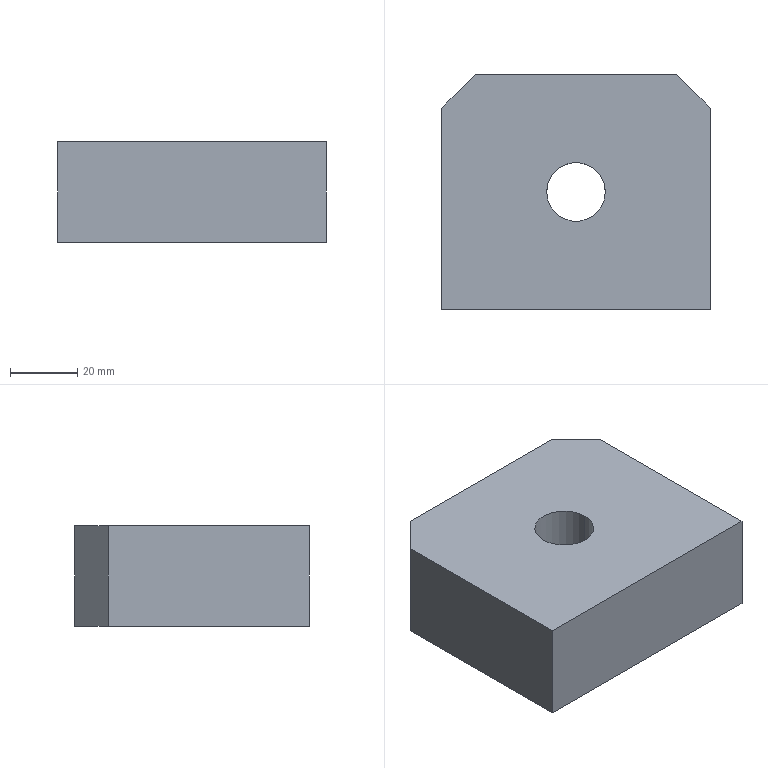Part | STEP file | Thickening Block | 1 solid | 10 faces | box 80 x 70 x 30 mm | volume 157784 mm3 | plane 8 | cylinder 2 | commonest cylinder face diameters 17.5 x2
STEP:
#1=CARTESIAN_POINT('',(0.,0.,0.));
#2=DIRECTION('',(0.,0.,1.));
#3=DIRECTION('',(1.,0.,0.));
#4=AXIS2_PLACEMENT_3D('',#1,#2,#3);
#5=CARTESIAN_POINT('',(8.75,0.,0.));
#6=VERTEX_POINT('',#5);
#7=CARTESIAN_POINT('',(8.75,0.,30.));
#8=VERTEX_POINT('',#7);
#9=CARTESIAN_POINT('',(8.75,0.,30.));
#10=DIRECTION('',(0.,0.,1.));
#11=VECTOR('',#10,1.);
#12=LINE('',#9,#11);
#13=CARTESIAN_POINT('',(0.,0.,30.));
#14=DIRECTION('',(0.,0.,1.));
#15=DIRECTION('',(1.,0.,0.));
#16=AXIS2_PLACEMENT_3D('',#13,#14,#15);
#17=CYLINDRICAL_SURFACE('',#16,8.75);
#18=CARTESIAN_POINT('',(6.283,0.));
#19=DIRECTION('',(0.,1.));
#20=VECTOR('',#19,1.);
#21=LINE('',#18,#20);
#22=(GEOMETRIC_REPRESENTATION_CONTEXT(2)PARAMETRIC_REPRESENTATION_CONTEXT()REPRESENTATION_CONTEXT('',''));
#23=DEFINITIONAL_REPRESENTATION('',(#21),#22);
#24=PCURVE('',#17,#23);
#25=CARTESIAN_POINT('',(0.,0.,30.));
#26=DIRECTION('',(0.,0.,1.));
#27=DIRECTION('',(1.,0.,0.));
#28=AXIS2_PLACEMENT_3D('',#25,#26,#27);
#29=CYLINDRICAL_SURFACE('',#28,8.75);
#30=CARTESIAN_POINT('',(0.,0.));
#31=DIRECTION('',(0.,1.));
#32=VECTOR('',#31,1.);
#33=LINE('',#30,#32);
#34=(GEOMETRIC_REPRESENTATION_CONTEXT(2)PARAMETRIC_REPRESENTATION_CONTEXT()REPRESENTATION_CONTEXT('',''));
#35=DEFINITIONAL_REPRESENTATION('',(#33),#34);
#36=PCURVE('',#29,#35);
#37=SURFACE_CURVE('',#12,(#24,#36),.PCURVE_S1.);
#38=EDGE_CURVE('',#6,#8,#37,.T.);
#39=ORIENTED_EDGE('',*,*,#38,.T.);
#40=CARTESIAN_POINT('',(-8.75,0.,30.));
#41=VERTEX_POINT('',#40);
#42=CARTESIAN_POINT('',(0.,0.,30.));
#43=DIRECTION('',(0.,0.,1.));
#44=DIRECTION('',(1.,0.,0.));
#45=AXIS2_PLACEMENT_3D('',#42,#43,#44);
#46=CIRCLE('',#45,8.75);
#47=CARTESIAN_POINT('',(0.,0.));
#48=DIRECTION('',(1.,0.));
#49=VECTOR('',#48,1.);
#50=LINE('',#47,#49);
#51=(GEOMETRIC_REPRESENTATION_CONTEXT(2)PARAMETRIC_REPRESENTATION_CONTEXT()REPRESENTATION_CONTEXT('',''));
#52=DEFINITIONAL_REPRESENTATION('',(#50),#51);
#53=PCURVE('',#17,#52);
#54=CARTESIAN_POINT('',(0.,0.,30.));
#55=DIRECTION('',(0.,0.,1.));
#56=DIRECTION('',(1.,0.,0.));
#57=AXIS2_PLACEMENT_3D('',#54,#55,#56);
#58=PLANE('',#57);
#59=CARTESIAN_POINT('',(0.,0.));
#60=DIRECTION('',(1.,0.));
#61=AXIS2_PLACEMENT_2D('',#59,#60);
#62=CIRCLE('',#61,8.75);
#63=(GEOMETRIC_REPRESENTATION_CONTEXT(2)PARAMETRIC_REPRESENTATION_CONTEXT()REPRESENTATION_CONTEXT('',''));
#64=DEFINITIONAL_REPRESENTATION('',(#62),#63);
#65=PCURVE('',#58,#64);
#66=SURFACE_CURVE('',#46,(#53,#65),.PCURVE_S1.);
#67=EDGE_CURVE('',#41,#8,#66,.T.);
#68=ORIENTED_EDGE('',*,*,#67,.F.);
#69=CARTESIAN_POINT('',(-8.75,0.,0.));
#70=VERTEX_POINT('',#69);
#71=CARTESIAN_POINT('',(-8.75,0.,30.));
#72=DIRECTION('',(0.,0.,1.));
#73=VECTOR('',#72,1.);
#74=LINE('',#71,#73);
#75=CARTESIAN_POINT('',(3.142,0.));
#76=DIRECTION('',(0.,1.));
#77=VECTOR('',#76,1.);
#78=LINE('',#75,#77);
#79=(GEOMETRIC_REPRESENTATION_CONTEXT(2)PARAMETRIC_REPRESENTATION_CONTEXT()REPRESENTATION_CONTEXT('',''));
#80=DEFINITIONAL_REPRESENTATION('',(#78),#79);
#81=PCURVE('',#17,#80);
#82=CARTESIAN_POINT('',(3.142,0.));
#83=DIRECTION('',(0.,1.));
#84=VECTOR('',#83,1.);
#85=LINE('',#82,#84);
#86=(GEOMETRIC_REPRESENTATION_CONTEXT(2)PARAMETRIC_REPRESENTATION_CONTEXT()REPRESENTATION_CONTEXT('',''));
#87=DEFINITIONAL_REPRESENTATION('',(#85),#86);
#88=PCURVE('',#29,#87);
#89=SURFACE_CURVE('',#74,(#81,#88),.PCURVE_S1.);
#90=EDGE_CURVE('',#70,#41,#89,.T.);
#91=ORIENTED_EDGE('',*,*,#90,.F.);
#92=CARTESIAN_POINT('',(0.,0.,0.));
#93=DIRECTION('',(0.,0.,1.));
#94=DIRECTION('',(1.,0.,0.));
#95=AXIS2_PLACEMENT_3D('',#92,#93,#94);
#96=CIRCLE('',#95,8.75);
#97=CARTESIAN_POINT('',(0.,-30.));
#98=DIRECTION('',(1.,0.));
#99=VECTOR('',#98,1.);
#100=LINE('',#97,#99);
#101=(GEOMETRIC_REPRESENTATION_CONTEXT(2)PARAMETRIC_REPRESENTATION_CONTEXT()REPRESENTATION_CONTEXT('',''));
#102=DEFINITIONAL_REPRESENTATION('',(#100),#101);
#103=PCURVE('',#17,#102);
#104=CARTESIAN_POINT('',(0.,0.,0.));
#105=DIRECTION('',(0.,0.,1.));
#106=DIRECTION('',(1.,0.,0.));
#107=AXIS2_PLACEMENT_3D('',#104,#105,#106);
#108=PLANE('',#107);
#109=CARTESIAN_POINT('',(0.,0.));
#110=DIRECTION('',(1.,0.));
#111=AXIS2_PLACEMENT_2D('',#109,#110);
#112=CIRCLE('',#111,8.75);
#113=(GEOMETRIC_REPRESENTATION_CONTEXT(2)PARAMETRIC_REPRESENTATION_CONTEXT()REPRESENTATION_CONTEXT('',''));
#114=DEFINITIONAL_REPRESENTATION('',(#112),#113);
#115=PCURVE('',#108,#114);
#116=SURFACE_CURVE('',#96,(#103,#115),.PCURVE_S1.);
#117=EDGE_CURVE('',#70,#6,#116,.T.);
#118=ORIENTED_EDGE('',*,*,#117,.T.);
#119=EDGE_LOOP('',(#39,#68,#91,#118));
#120=FACE_BOUND('',#119,.F.);
#121=ADVANCED_FACE('',(#120),#17,.F.);
#122=CARTESIAN_POINT('',(40.,-35.,0.));
#123=VERTEX_POINT('',#122);
#124=CARTESIAN_POINT('',(40.,25.,0.));
#125=VERTEX_POINT('',#124);
#126=CARTESIAN_POINT('',(40.,35.,0.));
#127=DIRECTION('',(0.,1.,0.));
#128=VECTOR('',#127,1.);
#129=LINE('',#126,#128);
#130=CARTESIAN_POINT('',(40.,35.,30.));
#131=DIRECTION('',(-1.,0.,0.));
#132=DIRECTION('',(0.,-1.,0.));
#133=AXIS2_PLACEMENT_3D('',#130,#131,#132);
#134=PLANE('',#133);
#135=CARTESIAN_POINT('',(0.,-30.));
#136=DIRECTION('',(-1.,0.));
#137=VECTOR('',#136,1.);
#138=LINE('',#135,#137);
#139=(GEOMETRIC_REPRESENTATION_CONTEXT(2)PARAMETRIC_REPRESENTATION_CONTEXT()REPRESENTATION_CONTEXT('',''));
#140=DEFINITIONAL_REPRESENTATION('',(#138),#139);
#141=PCURVE('',#134,#140);
#142=CARTESIAN_POINT('',(40.,35.));
#143=DIRECTION('',(0.,1.));
#144=VECTOR('',#143,1.);
#145=LINE('',#142,#144);
#146=(GEOMETRIC_REPRESENTATION_CONTEXT(2)PARAMETRIC_REPRESENTATION_CONTEXT()REPRESENTATION_CONTEXT('',''));
#147=DEFINITIONAL_REPRESENTATION('',(#145),#146);
#148=PCURVE('',#108,#147);
#149=SURFACE_CURVE('',#129,(#141,#148),.PCURVE_S1.);
#150=EDGE_CURVE('',#123,#125,#149,.T.);
#151=ORIENTED_EDGE('',*,*,#150,.T.);
#152=CARTESIAN_POINT('',(40.,25.,30.));
#153=VERTEX_POINT('',#152);
#154=CARTESIAN_POINT('',(40.,25.,30.));
#155=DIRECTION('',(0.,0.,1.));
#156=VECTOR('',#155,1.);
#157=LINE('',#154,#156);
#158=CARTESIAN_POINT('',(10.,0.));
#159=DIRECTION('',(0.,1.));
#160=VECTOR('',#159,1.);
#161=LINE('',#158,#160);
#162=(GEOMETRIC_REPRESENTATION_CONTEXT(2)PARAMETRIC_REPRESENTATION_CONTEXT()REPRESENTATION_CONTEXT('',''));
#163=DEFINITIONAL_REPRESENTATION('',(#161),#162);
#164=PCURVE('',#134,#163);
#165=CARTESIAN_POINT('',(30.,35.,30.));
#166=DIRECTION('',(-0.7071,-0.7071,0.));
#167=DIRECTION('',(0.,0.,-1.));
#168=AXIS2_PLACEMENT_3D('',#165,#166,#167);
#169=PLANE('',#168);
#170=CARTESIAN_POINT('',(0.,14.142));
#171=DIRECTION('',(-1.,0.));
#172=VECTOR('',#171,1.);
#173=LINE('',#170,#172);
#174=(GEOMETRIC_REPRESENTATION_CONTEXT(2)PARAMETRIC_REPRESENTATION_CONTEXT()REPRESENTATION_CONTEXT('',''));
#175=DEFINITIONAL_REPRESENTATION('',(#173),#174);
#176=PCURVE('',#169,#175);
#177=SURFACE_CURVE('',#157,(#164,#176),.PCURVE_S1.);
#178=EDGE_CURVE('',#125,#153,#177,.T.);
#179=ORIENTED_EDGE('',*,*,#178,.T.);
#180=CARTESIAN_POINT('',(40.,-35.,30.));
#181=VERTEX_POINT('',#180);
#182=CARTESIAN_POINT('',(40.,35.,30.));
#183=DIRECTION('',(0.,1.,0.));
#184=VECTOR('',#183,1.);
#185=LINE('',#182,#184);
#186=CARTESIAN_POINT('',(0.,0.));
#187=DIRECTION('',(-1.,0.));
#188=VECTOR('',#187,1.);
#189=LINE('',#186,#188);
#190=(GEOMETRIC_REPRESENTATION_CONTEXT(2)PARAMETRIC_REPRESENTATION_CONTEXT()REPRESENTATION_CONTEXT('',''));
#191=DEFINITIONAL_REPRESENTATION('',(#189),#190);
#192=PCURVE('',#134,#191);
#193=CARTESIAN_POINT('',(40.,35.));
#194=DIRECTION('',(0.,1.));
#195=VECTOR('',#194,1.);
#196=LINE('',#193,#195);
#197=(GEOMETRIC_REPRESENTATION_CONTEXT(2)PARAMETRIC_REPRESENTATION_CONTEXT()REPRESENTATION_CONTEXT('',''));
#198=DEFINITIONAL_REPRESENTATION('',(#196),#197);
#199=PCURVE('',#58,#198);
#200=SURFACE_CURVE('',#185,(#192,#199),.PCURVE_S1.);
#201=EDGE_CURVE('',#181,#153,#200,.T.);
#202=ORIENTED_EDGE('',*,*,#201,.F.);
#203=CARTESIAN_POINT('',(40.,-35.,30.));
#204=DIRECTION('',(0.,0.,-1.));
#205=VECTOR('',#204,1.);
#206=LINE('',#203,#205);
#207=CARTESIAN_POINT('',(70.,0.));
#208=DIRECTION('',(0.,-1.));
#209=VECTOR('',#208,1.);
#210=LINE('',#207,#209);
#211=(GEOMETRIC_REPRESENTATION_CONTEXT(2)PARAMETRIC_REPRESENTATION_CONTEXT()REPRESENTATION_CONTEXT('',''));
#212=DEFINITIONAL_REPRESENTATION('',(#210),#211);
#213=PCURVE('',#134,#212);
#214=CARTESIAN_POINT('',(-40.,-35.,30.));
#215=DIRECTION('',(0.,1.,0.));
#216=DIRECTION('',(0.,0.,1.));
#217=AXIS2_PLACEMENT_3D('',#214,#215,#216);
#218=PLANE('',#217);
#219=CARTESIAN_POINT('',(0.,80.));
#220=DIRECTION('',(-1.,0.));
#221=VECTOR('',#220,1.);
#222=LINE('',#219,#221);
#223=(GEOMETRIC_REPRESENTATION_CONTEXT(2)PARAMETRIC_REPRESENTATION_CONTEXT()REPRESENTATION_CONTEXT('',''));
#224=DEFINITIONAL_REPRESENTATION('',(#222),#223);
#225=PCURVE('',#218,#224);
#226=SURFACE_CURVE('',#206,(#213,#225),.PCURVE_S1.);
#227=EDGE_CURVE('',#181,#123,#226,.T.);
#228=ORIENTED_EDGE('',*,*,#227,.T.);
#229=EDGE_LOOP('',(#151,#179,#202,#228));
#230=FACE_BOUND('',#229,.T.);
#231=ADVANCED_FACE('',(#230),#134,.F.);
#232=CARTESIAN_POINT('',(30.,35.,30.));
#233=VERTEX_POINT('',#232);
#234=CARTESIAN_POINT('',(-30.,35.,30.));
#235=VERTEX_POINT('',#234);
#236=CARTESIAN_POINT('',(-40.,35.,30.));
#237=DIRECTION('',(-1.,0.,0.));
#238=VECTOR('',#237,1.);
#239=LINE('',#236,#238);
#240=CARTESIAN_POINT('',(-40.,35.,30.));
#241=DIRECTION('',(0.,-1.,0.));
#242=DIRECTION('',(0.,0.,-1.));
#243=AXIS2_PLACEMENT_3D('',#240,#241,#242);
#244=PLANE('',#243);
#245=CARTESIAN_POINT('',(0.,0.));
#246=DIRECTION('',(0.,-1.));
#247=VECTOR('',#246,1.);
#248=LINE('',#245,#247);
#249=(GEOMETRIC_REPRESENTATION_CONTEXT(2)PARAMETRIC_REPRESENTATION_CONTEXT()REPRESENTATION_CONTEXT('',''));
#250=DEFINITIONAL_REPRESENTATION('',(#248),#249);
#251=PCURVE('',#244,#250);
#252=CARTESIAN_POINT('',(-40.,35.));
#253=DIRECTION('',(-1.,0.));
#254=VECTOR('',#253,1.);
#255=LINE('',#252,#254);
#256=(GEOMETRIC_REPRESENTATION_CONTEXT(2)PARAMETRIC_REPRESENTATION_CONTEXT()REPRESENTATION_CONTEXT('',''));
#257=DEFINITIONAL_REPRESENTATION('',(#255),#256);
#258=PCURVE('',#58,#257);
#259=SURFACE_CURVE('',#239,(#251,#258),.PCURVE_S1.);
#260=EDGE_CURVE('',#233,#235,#259,.T.);
#261=ORIENTED_EDGE('',*,*,#260,.F.);
#262=CARTESIAN_POINT('',(30.,35.,0.));
#263=VERTEX_POINT('',#262);
#264=CARTESIAN_POINT('',(30.,35.,30.));
#265=DIRECTION('',(0.,0.,-1.));
#266=VECTOR('',#265,1.);
#267=LINE('',#264,#266);
#268=CARTESIAN_POINT('',(0.,70.));
#269=DIRECTION('',(1.,0.));
#270=VECTOR('',#269,1.);
#271=LINE('',#268,#270);
#272=(GEOMETRIC_REPRESENTATION_CONTEXT(2)PARAMETRIC_REPRESENTATION_CONTEXT()REPRESENTATION_CONTEXT('',''));
#273=DEFINITIONAL_REPRESENTATION('',(#271),#272);
#274=PCURVE('',#244,#273);
#275=CARTESIAN_POINT('',(0.,0.));
#276=DIRECTION('',(1.,0.));
#277=VECTOR('',#276,1.);
#278=LINE('',#275,#277);
#279=(GEOMETRIC_REPRESENTATION_CONTEXT(2)PARAMETRIC_REPRESENTATION_CONTEXT()REPRESENTATION_CONTEXT('',''));
#280=DEFINITIONAL_REPRESENTATION('',(#278),#279);
#281=PCURVE('',#169,#280);
#282=SURFACE_CURVE('',#267,(#274,#281),.PCURVE_S1.);
#283=EDGE_CURVE('',#233,#263,#282,.T.);
#284=ORIENTED_EDGE('',*,*,#283,.T.);
#285=CARTESIAN_POINT('',(-30.,35.,0.));
#286=VERTEX_POINT('',#285);
#287=CARTESIAN_POINT('',(-40.,35.,0.));
#288=DIRECTION('',(-1.,0.,0.));
#289=VECTOR('',#288,1.);
#290=LINE('',#287,#289);
#291=CARTESIAN_POINT('',(30.,0.));
#292=DIRECTION('',(0.,-1.));
#293=VECTOR('',#292,1.);
#294=LINE('',#291,#293);
#295=(GEOMETRIC_REPRESENTATION_CONTEXT(2)PARAMETRIC_REPRESENTATION_CONTEXT()REPRESENTATION_CONTEXT('',''));
#296=DEFINITIONAL_REPRESENTATION('',(#294),#295);
#297=PCURVE('',#244,#296);
#298=CARTESIAN_POINT('',(-40.,35.));
#299=DIRECTION('',(-1.,0.));
#300=VECTOR('',#299,1.);
#301=LINE('',#298,#300);
#302=(GEOMETRIC_REPRESENTATION_CONTEXT(2)PARAMETRIC_REPRESENTATION_CONTEXT()REPRESENTATION_CONTEXT('',''));
#303=DEFINITIONAL_REPRESENTATION('',(#301),#302);
#304=PCURVE('',#108,#303);
#305=SURFACE_CURVE('',#290,(#297,#304),.PCURVE_S1.);
#306=EDGE_CURVE('',#263,#286,#305,.T.);
#307=ORIENTED_EDGE('',*,*,#306,.T.);
#308=CARTESIAN_POINT('',(-30.,35.,30.));
#309=DIRECTION('',(0.,0.,1.));
#310=VECTOR('',#309,1.);
#311=LINE('',#308,#310);
#312=CARTESIAN_POINT('',(0.,10.));
#313=DIRECTION('',(-1.,0.));
#314=VECTOR('',#313,1.);
#315=LINE('',#312,#314);
#316=(GEOMETRIC_REPRESENTATION_CONTEXT(2)PARAMETRIC_REPRESENTATION_CONTEXT()REPRESENTATION_CONTEXT('',''));
#317=DEFINITIONAL_REPRESENTATION('',(#315),#316);
#318=PCURVE('',#244,#317);
#319=CARTESIAN_POINT('',(-40.,25.,30.));
#320=DIRECTION('',(0.7071,-0.7071,0.));
#321=DIRECTION('',(0.,0.,-1.));
#322=AXIS2_PLACEMENT_3D('',#319,#320,#321);
#323=PLANE('',#322);
#324=CARTESIAN_POINT('',(0.,14.142));
#325=DIRECTION('',(-1.,0.));
#326=VECTOR('',#325,1.);
#327=LINE('',#324,#326);
#328=(GEOMETRIC_REPRESENTATION_CONTEXT(2)PARAMETRIC_REPRESENTATION_CONTEXT()REPRESENTATION_CONTEXT('',''));
#329=DEFINITIONAL_REPRESENTATION('',(#327),#328);
#330=PCURVE('',#323,#329);
#331=SURFACE_CURVE('',#311,(#318,#330),.PCURVE_S1.);
#332=EDGE_CURVE('',#286,#235,#331,.T.);
#333=ORIENTED_EDGE('',*,*,#332,.T.);
#334=EDGE_LOOP('',(#261,#284,#307,#333));
#335=FACE_BOUND('',#334,.T.);
#336=ADVANCED_FACE('',(#335),#244,.F.);
#337=CARTESIAN_POINT('',(-40.,25.,30.));
#338=VERTEX_POINT('',#337);
#339=CARTESIAN_POINT('',(-40.,-35.,30.));
#340=VERTEX_POINT('',#339);
#341=CARTESIAN_POINT('',(-40.,35.,30.));
#342=DIRECTION('',(0.,-1.,0.));
#343=VECTOR('',#342,1.);
#344=LINE('',#341,#343);
#345=CARTESIAN_POINT('',(-40.,35.,30.));
#346=DIRECTION('',(1.,0.,0.));
#347=DIRECTION('',(0.,1.,0.));
#348=AXIS2_PLACEMENT_3D('',#345,#346,#347);
#349=PLANE('',#348);
#350=CARTESIAN_POINT('',(0.,0.));
#351=DIRECTION('',(-1.,0.));
#352=VECTOR('',#351,1.);
#353=LINE('',#350,#352);
#354=(GEOMETRIC_REPRESENTATION_CONTEXT(2)PARAMETRIC_REPRESENTATION_CONTEXT()REPRESENTATION_CONTEXT('',''));
#355=DEFINITIONAL_REPRESENTATION('',(#353),#354);
#356=PCURVE('',#349,#355);
#357=CARTESIAN_POINT('',(-40.,35.));
#358=DIRECTION('',(0.,-1.));
#359=VECTOR('',#358,1.);
#360=LINE('',#357,#359);
#361=(GEOMETRIC_REPRESENTATION_CONTEXT(2)PARAMETRIC_REPRESENTATION_CONTEXT()REPRESENTATION_CONTEXT('',''));
#362=DEFINITIONAL_REPRESENTATION('',(#360),#361);
#363=PCURVE('',#58,#362);
#364=SURFACE_CURVE('',#344,(#356,#363),.PCURVE_S1.);
#365=EDGE_CURVE('',#338,#340,#364,.T.);
#366=ORIENTED_EDGE('',*,*,#365,.F.);
#367=CARTESIAN_POINT('',(-40.,25.,0.));
#368=VERTEX_POINT('',#367);
#369=CARTESIAN_POINT('',(-40.,25.,30.));
#370=DIRECTION('',(0.,0.,-1.));
#371=VECTOR('',#370,1.);
#372=LINE('',#369,#371);
#373=CARTESIAN_POINT('',(-10.,0.));
#374=DIRECTION('',(0.,-1.));
#375=VECTOR('',#374,1.);
#376=LINE('',#373,#375);
#377=(GEOMETRIC_REPRESENTATION_CONTEXT(2)PARAMETRIC_REPRESENTATION_CONTEXT()REPRESENTATION_CONTEXT('',''));
#378=DEFINITIONAL_REPRESENTATION('',(#376),#377);
#379=PCURVE('',#349,#378);
#380=CARTESIAN_POINT('',(0.,0.));
#381=DIRECTION('',(1.,0.));
#382=VECTOR('',#381,1.);
#383=LINE('',#380,#382);
#384=(GEOMETRIC_REPRESENTATION_CONTEXT(2)PARAMETRIC_REPRESENTATION_CONTEXT()REPRESENTATION_CONTEXT('',''));
#385=DEFINITIONAL_REPRESENTATION('',(#383),#384);
#386=PCURVE('',#323,#385);
#387=SURFACE_CURVE('',#372,(#379,#386),.PCURVE_S1.);
#388=EDGE_CURVE('',#338,#368,#387,.T.);
#389=ORIENTED_EDGE('',*,*,#388,.T.);
#390=CARTESIAN_POINT('',(-40.,-35.,0.));
#391=VERTEX_POINT('',#390);
#392=CARTESIAN_POINT('',(-40.,35.,0.));
#393=DIRECTION('',(0.,-1.,0.));
#394=VECTOR('',#393,1.);
#395=LINE('',#392,#394);
#396=CARTESIAN_POINT('',(0.,-30.));
#397=DIRECTION('',(-1.,0.));
#398=VECTOR('',#397,1.);
#399=LINE('',#396,#398);
#400=(GEOMETRIC_REPRESENTATION_CONTEXT(2)PARAMETRIC_REPRESENTATION_CONTEXT()REPRESENTATION_CONTEXT('',''));
#401=DEFINITIONAL_REPRESENTATION('',(#399),#400);
#402=PCURVE('',#349,#401);
#403=CARTESIAN_POINT('',(-40.,35.));
#404=DIRECTION('',(0.,-1.));
#405=VECTOR('',#404,1.);
#406=LINE('',#403,#405);
#407=(GEOMETRIC_REPRESENTATION_CONTEXT(2)PARAMETRIC_REPRESENTATION_CONTEXT()REPRESENTATION_CONTEXT('',''));
#408=DEFINITIONAL_REPRESENTATION('',(#406),#407);
#409=PCURVE('',#108,#408);
#410=SURFACE_CURVE('',#395,(#402,#409),.PCURVE_S1.);
#411=EDGE_CURVE('',#368,#391,#410,.T.);
#412=ORIENTED_EDGE('',*,*,#411,.T.);
#413=CARTESIAN_POINT('',(-40.,-35.,30.));
#414=DIRECTION('',(0.,0.,-1.));
#415=VECTOR('',#414,1.);
#416=LINE('',#413,#415);
#417=CARTESIAN_POINT('',(-70.,0.));
#418=DIRECTION('',(0.,-1.));
#419=VECTOR('',#418,1.);
#420=LINE('',#417,#419);
#421=(GEOMETRIC_REPRESENTATION_CONTEXT(2)PARAMETRIC_REPRESENTATION_CONTEXT()REPRESENTATION_CONTEXT('',''));
#422=DEFINITIONAL_REPRESENTATION('',(#420),#421);
#423=PCURVE('',#349,#422);
#424=CARTESIAN_POINT('',(0.,0.));
#425=DIRECTION('',(-1.,0.));
#426=VECTOR('',#425,1.);
#427=LINE('',#424,#426);
#428=(GEOMETRIC_REPRESENTATION_CONTEXT(2)PARAMETRIC_REPRESENTATION_CONTEXT()REPRESENTATION_CONTEXT('',''));
#429=DEFINITIONAL_REPRESENTATION('',(#427),#428);
#430=PCURVE('',#218,#429);
#431=SURFACE_CURVE('',#416,(#423,#430),.PCURVE_S1.);
#432=EDGE_CURVE('',#340,#391,#431,.T.);
#433=ORIENTED_EDGE('',*,*,#432,.F.);
#434=EDGE_LOOP('',(#366,#389,#412,#433));
#435=FACE_BOUND('',#434,.T.);
#436=ADVANCED_FACE('',(#435),#349,.F.);
#437=CARTESIAN_POINT('',(-40.,-35.,0.));
#438=DIRECTION('',(1.,0.,0.));
#439=VECTOR('',#438,1.);
#440=LINE('',#437,#439);
#441=CARTESIAN_POINT('',(-30.,0.));
#442=DIRECTION('',(0.,1.));
#443=VECTOR('',#442,1.);
#444=LINE('',#441,#443);
#445=(GEOMETRIC_REPRESENTATION_CONTEXT(2)PARAMETRIC_REPRESENTATION_CONTEXT()REPRESENTATION_CONTEXT('',''));
#446=DEFINITIONAL_REPRESENTATION('',(#444),#445);
#447=PCURVE('',#218,#446);
#448=CARTESIAN_POINT('',(-40.,-35.));
#449=DIRECTION('',(1.,0.));
#450=VECTOR('',#449,1.);
#451=LINE('',#448,#450);
#452=(GEOMETRIC_REPRESENTATION_CONTEXT(2)PARAMETRIC_REPRESENTATION_CONTEXT()REPRESENTATION_CONTEXT('',''));
#453=DEFINITIONAL_REPRESENTATION('',(#451),#452);
#454=PCURVE('',#108,#453);
#455=SURFACE_CURVE('',#440,(#447,#454),.PCURVE_S1.);
#456=EDGE_CURVE('',#391,#123,#455,.T.);
#457=ORIENTED_EDGE('',*,*,#456,.T.);
#458=ORIENTED_EDGE('',*,*,#227,.F.);
#459=CARTESIAN_POINT('',(-40.,-35.,30.));
#460=DIRECTION('',(1.,0.,0.));
#461=VECTOR('',#460,1.);
#462=LINE('',#459,#461);
#463=CARTESIAN_POINT('',(0.,0.));
#464=DIRECTION('',(0.,1.));
#465=VECTOR('',#464,1.);
#466=LINE('',#463,#465);
#467=(GEOMETRIC_REPRESENTATION_CONTEXT(2)PARAMETRIC_REPRESENTATION_CONTEXT()REPRESENTATION_CONTEXT('',''));
#468=DEFINITIONAL_REPRESENTATION('',(#466),#467);
#469=PCURVE('',#218,#468);
#470=CARTESIAN_POINT('',(-40.,-35.));
#471=DIRECTION('',(1.,0.));
#472=VECTOR('',#471,1.);
#473=LINE('',#470,#472);
#474=(GEOMETRIC_REPRESENTATION_CONTEXT(2)PARAMETRIC_REPRESENTATION_CONTEXT()REPRESENTATION_CONTEXT('',''));
#475=DEFINITIONAL_REPRESENTATION('',(#473),#474);
#476=PCURVE('',#58,#475);
#477=SURFACE_CURVE('',#462,(#469,#476),.PCURVE_S1.);
#478=EDGE_CURVE('',#340,#181,#477,.T.);
#479=ORIENTED_EDGE('',*,*,#478,.F.);
#480=ORIENTED_EDGE('',*,*,#432,.T.);
#481=EDGE_LOOP('',(#457,#458,#479,#480));
#482=FACE_BOUND('',#481,.T.);
#483=ADVANCED_FACE('',(#482),#218,.F.);
#484=CARTESIAN_POINT('',(0.,0.,30.));
#485=DIRECTION('',(0.,0.,1.));
#486=DIRECTION('',(1.,0.,0.));
#487=AXIS2_PLACEMENT_3D('',#484,#485,#486);
#488=CIRCLE('',#487,8.75);
#489=CARTESIAN_POINT('',(0.,0.));
#490=DIRECTION('',(1.,0.));
#491=AXIS2_PLACEMENT_2D('',#489,#490);
#492=CIRCLE('',#491,8.75);
#493=(GEOMETRIC_REPRESENTATION_CONTEXT(2)PARAMETRIC_REPRESENTATION_CONTEXT()REPRESENTATION_CONTEXT('',''));
#494=DEFINITIONAL_REPRESENTATION('',(#492),#493);
#495=PCURVE('',#58,#494);
#496=CARTESIAN_POINT('',(0.,0.));
#497=DIRECTION('',(1.,0.));
#498=VECTOR('',#497,1.);
#499=LINE('',#496,#498);
#500=(GEOMETRIC_REPRESENTATION_CONTEXT(2)PARAMETRIC_REPRESENTATION_CONTEXT()REPRESENTATION_CONTEXT('',''));
#501=DEFINITIONAL_REPRESENTATION('',(#499),#500);
#502=PCURVE('',#29,#501);
#503=SURFACE_CURVE('',#488,(#495,#502),.PCURVE_S1.);
#504=EDGE_CURVE('',#8,#41,#503,.T.);
#505=ORIENTED_EDGE('',*,*,#504,.F.);
#506=ORIENTED_EDGE('',*,*,#67,.F.);
#507=EDGE_LOOP('',(#505,#506));
#508=FACE_BOUND('',#507,.T.);
#509=ORIENTED_EDGE('',*,*,#201,.T.);
#510=CARTESIAN_POINT('',(32.5,32.5,30.));
#511=DIRECTION('',(-0.7071,0.7071,0.));
#512=VECTOR('',#511,1.);
#513=LINE('',#510,#512);
#514=CARTESIAN_POINT('',(32.5,32.5));
#515=DIRECTION('',(-0.7071,0.7071));
#516=VECTOR('',#515,1.);
#517=LINE('',#514,#516);
#518=(GEOMETRIC_REPRESENTATION_CONTEXT(2)PARAMETRIC_REPRESENTATION_CONTEXT()REPRESENTATION_CONTEXT('',''));
#519=DEFINITIONAL_REPRESENTATION('',(#517),#518);
#520=PCURVE('',#58,#519);
#521=CARTESIAN_POINT('',(0.,3.536));
#522=DIRECTION('',(0.,-1.));
#523=VECTOR('',#522,1.);
#524=LINE('',#521,#523);
#525=(GEOMETRIC_REPRESENTATION_CONTEXT(2)PARAMETRIC_REPRESENTATION_CONTEXT()REPRESENTATION_CONTEXT('',''));
#526=DEFINITIONAL_REPRESENTATION('',(#524),#525);
#527=PCURVE('',#169,#526);
#528=SURFACE_CURVE('',#513,(#520,#527),.PCURVE_S1.);
#529=EDGE_CURVE('',#153,#233,#528,.T.);
#530=ORIENTED_EDGE('',*,*,#529,.T.);
#531=ORIENTED_EDGE('',*,*,#260,.T.);
#532=CARTESIAN_POINT('',(-32.5,32.5,30.));
#533=DIRECTION('',(-0.7071,-0.7071,0.));
#534=VECTOR('',#533,1.);
#535=LINE('',#532,#534);
#536=CARTESIAN_POINT('',(-32.5,32.5));
#537=DIRECTION('',(-0.7071,-0.7071));
#538=VECTOR('',#537,1.);
#539=LINE('',#536,#538);
#540=(GEOMETRIC_REPRESENTATION_CONTEXT(2)PARAMETRIC_REPRESENTATION_CONTEXT()REPRESENTATION_CONTEXT('',''));
#541=DEFINITIONAL_REPRESENTATION('',(#539),#540);
#542=PCURVE('',#58,#541);
#543=CARTESIAN_POINT('',(0.,10.607));
#544=DIRECTION('',(0.,-1.));
#545=VECTOR('',#544,1.);
#546=LINE('',#543,#545);
#547=(GEOMETRIC_REPRESENTATION_CONTEXT(2)PARAMETRIC_REPRESENTATION_CONTEXT()REPRESENTATION_CONTEXT('',''));
#548=DEFINITIONAL_REPRESENTATION('',(#546),#547);
#549=PCURVE('',#323,#548);
#550=SURFACE_CURVE('',#535,(#542,#549),.PCURVE_S1.);
#551=EDGE_CURVE('',#235,#338,#550,.T.);
#552=ORIENTED_EDGE('',*,*,#551,.T.);
#553=ORIENTED_EDGE('',*,*,#365,.T.);
#554=ORIENTED_EDGE('',*,*,#478,.T.);
#555=EDGE_LOOP('',(#509,#530,#531,#552,#553,#554));
#556=FACE_BOUND('',#555,.T.);
#557=ADVANCED_FACE('',(#508,#556),#58,.T.);
#558=CARTESIAN_POINT('',(0.,0.,0.));
#559=DIRECTION('',(0.,0.,1.));
#560=DIRECTION('',(1.,0.,0.));
#561=AXIS2_PLACEMENT_3D('',#558,#559,#560);
#562=CIRCLE('',#561,8.75);
#563=CARTESIAN_POINT('',(0.,0.));
#564=DIRECTION('',(1.,0.));
#565=AXIS2_PLACEMENT_2D('',#563,#564);
#566=CIRCLE('',#565,8.75);
#567=(GEOMETRIC_REPRESENTATION_CONTEXT(2)PARAMETRIC_REPRESENTATION_CONTEXT()REPRESENTATION_CONTEXT('',''));
#568=DEFINITIONAL_REPRESENTATION('',(#566),#567);
#569=PCURVE('',#108,#568);
#570=CARTESIAN_POINT('',(0.,-30.));
#571=DIRECTION('',(1.,0.));
#572=VECTOR('',#571,1.);
#573=LINE('',#570,#572);
#574=(GEOMETRIC_REPRESENTATION_CONTEXT(2)PARAMETRIC_REPRESENTATION_CONTEXT()REPRESENTATION_CONTEXT('',''));
#575=DEFINITIONAL_REPRESENTATION('',(#573),#574);
#576=PCURVE('',#29,#575);
#577=SURFACE_CURVE('',#562,(#569,#576),.PCURVE_S1.);
#578=EDGE_CURVE('',#6,#70,#577,.T.);
#579=ORIENTED_EDGE('',*,*,#578,.T.);
#580=ORIENTED_EDGE('',*,*,#117,.T.);
#581=EDGE_LOOP('',(#579,#580));
#582=FACE_BOUND('',#581,.T.);
#583=ORIENTED_EDGE('',*,*,#306,.F.);
#584=CARTESIAN_POINT('',(30.,35.,0.));
#585=DIRECTION('',(0.7071,-0.7071,0.));
#586=VECTOR('',#585,1.);
#587=LINE('',#584,#586);
#588=CARTESIAN_POINT('',(30.,35.));
#589=DIRECTION('',(0.7071,-0.7071));
#590=VECTOR('',#589,1.);
#591=LINE('',#588,#590);
#592=(GEOMETRIC_REPRESENTATION_CONTEXT(2)PARAMETRIC_REPRESENTATION_CONTEXT()REPRESENTATION_CONTEXT('',''));
#593=DEFINITIONAL_REPRESENTATION('',(#591),#592);
#594=PCURVE('',#108,#593);
#595=CARTESIAN_POINT('',(30.,0.));
#596=DIRECTION('',(0.,1.));
#597=VECTOR('',#596,1.);
#598=LINE('',#595,#597);
#599=(GEOMETRIC_REPRESENTATION_CONTEXT(2)PARAMETRIC_REPRESENTATION_CONTEXT()REPRESENTATION_CONTEXT('',''));
#600=DEFINITIONAL_REPRESENTATION('',(#598),#599);
#601=PCURVE('',#169,#600);
#602=SURFACE_CURVE('',#587,(#594,#601),.PCURVE_S1.);
#603=EDGE_CURVE('',#263,#125,#602,.T.);
#604=ORIENTED_EDGE('',*,*,#603,.T.);
#605=ORIENTED_EDGE('',*,*,#150,.F.);
#606=ORIENTED_EDGE('',*,*,#456,.F.);
#607=ORIENTED_EDGE('',*,*,#411,.F.);
#608=CARTESIAN_POINT('',(-40.,25.,0.));
#609=DIRECTION('',(0.7071,0.7071,0.));
#610=VECTOR('',#609,1.);
#611=LINE('',#608,#610);
#612=CARTESIAN_POINT('',(-40.,25.));
#613=DIRECTION('',(0.7071,0.7071));
#614=VECTOR('',#613,1.);
#615=LINE('',#612,#614);
#616=(GEOMETRIC_REPRESENTATION_CONTEXT(2)PARAMETRIC_REPRESENTATION_CONTEXT()REPRESENTATION_CONTEXT('',''));
#617=DEFINITIONAL_REPRESENTATION('',(#615),#616);
#618=PCURVE('',#108,#617);
#619=CARTESIAN_POINT('',(30.,0.));
#620=DIRECTION('',(0.,1.));
#621=VECTOR('',#620,1.);
#622=LINE('',#619,#621);
#623=(GEOMETRIC_REPRESENTATION_CONTEXT(2)PARAMETRIC_REPRESENTATION_CONTEXT()REPRESENTATION_CONTEXT('',''));
#624=DEFINITIONAL_REPRESENTATION('',(#622),#623);
#625=PCURVE('',#323,#624);
#626=SURFACE_CURVE('',#611,(#618,#625),.PCURVE_S1.);
#627=EDGE_CURVE('',#368,#286,#626,.T.);
#628=ORIENTED_EDGE('',*,*,#627,.T.);
#629=EDGE_LOOP('',(#583,#604,#605,#606,#607,#628));
#630=FACE_BOUND('',#629,.T.);
#631=ADVANCED_FACE('',(#582,#630),#108,.F.);
#632=ORIENTED_EDGE('',*,*,#529,.F.);
#633=ORIENTED_EDGE('',*,*,#178,.F.);
#634=ORIENTED_EDGE('',*,*,#603,.F.);
#635=ORIENTED_EDGE('',*,*,#283,.F.);
#636=EDGE_LOOP('',(#632,#633,#634,#635));
#637=FACE_BOUND('',#636,.T.);
#638=ADVANCED_FACE('',(#637),#169,.F.);
#639=ORIENTED_EDGE('',*,*,#551,.F.);
#640=ORIENTED_EDGE('',*,*,#332,.F.);
#641=ORIENTED_EDGE('',*,*,#627,.F.);
#642=ORIENTED_EDGE('',*,*,#388,.F.);
#643=EDGE_LOOP('',(#639,#640,#641,#642));
#644=FACE_BOUND('',#643,.T.);
#645=ADVANCED_FACE('',(#644),#323,.F.);
#646=ORIENTED_EDGE('',*,*,#504,.F.);
#647=ORIENTED_EDGE('',*,*,#38,.F.);
#648=ORIENTED_EDGE('',*,*,#578,.T.);
#649=ORIENTED_EDGE('',*,*,#90,.T.);
#650=EDGE_LOOP('',(#646,#647,#648,#649));
#651=FACE_BOUND('',#650,.F.);
#652=ADVANCED_FACE('',(#651),#29,.F.);
#653=CLOSED_SHELL('',(#121,#231,#336,#436,#483,#557,#631,#638,#645,#652));
#654=MANIFOLD_SOLID_BREP('',#653);
#655=(LENGTH_UNIT()NAMED_UNIT(*)SI_UNIT(.MILLI.,.METRE.));
#656=UNCERTAINTY_MEASURE_WITH_UNIT(LENGTH_MEASURE(0.0000001),#655,'','');
#657=(NAMED_UNIT(*)PLANE_ANGLE_UNIT()SI_UNIT($,.RADIAN.));
#658=(NAMED_UNIT(*)SI_UNIT($,.STERADIAN.)SOLID_ANGLE_UNIT());
#659=(GEOMETRIC_REPRESENTATION_CONTEXT(3)GLOBAL_UNCERTAINTY_ASSIGNED_CONTEXT((#656))GLOBAL_UNIT_ASSIGNED_CONTEXT((#655,#657,#658))REPRESENTATION_CONTEXT('',''));
#660=ADVANCED_BREP_SHAPE_REPRESENTATION('',(#4,#654),#659);